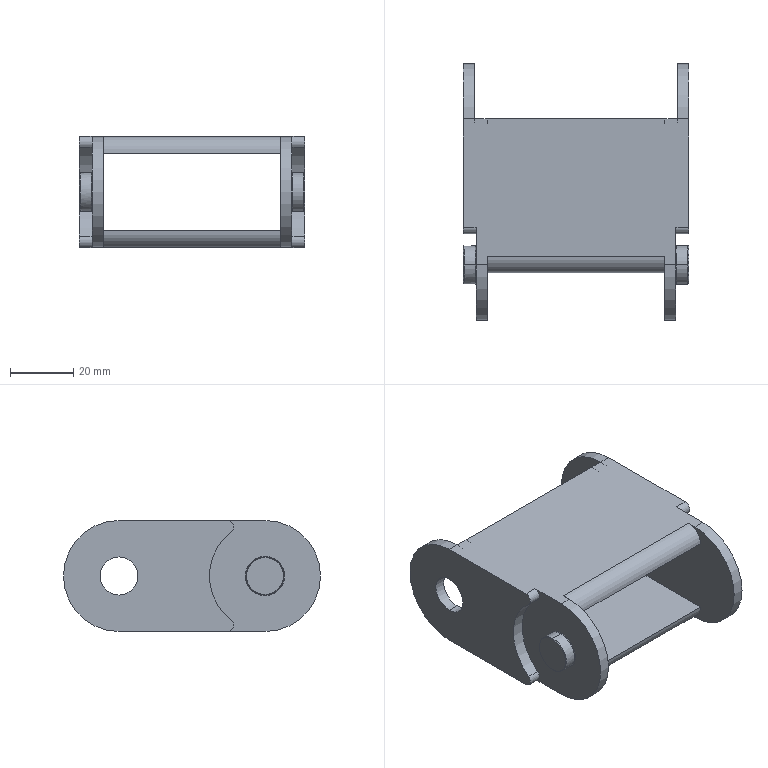Part | STEP file | TFH-CONNECTION57 | 1 solid | 50 faces | box 71 x 81 x 35 mm | volume 50324 mm3 | cylinder 24 | plane 18 | torus 6 | spline 2 | commonest cylinder face diameters 12 x8 35 x8 4 x4 10.5 x4